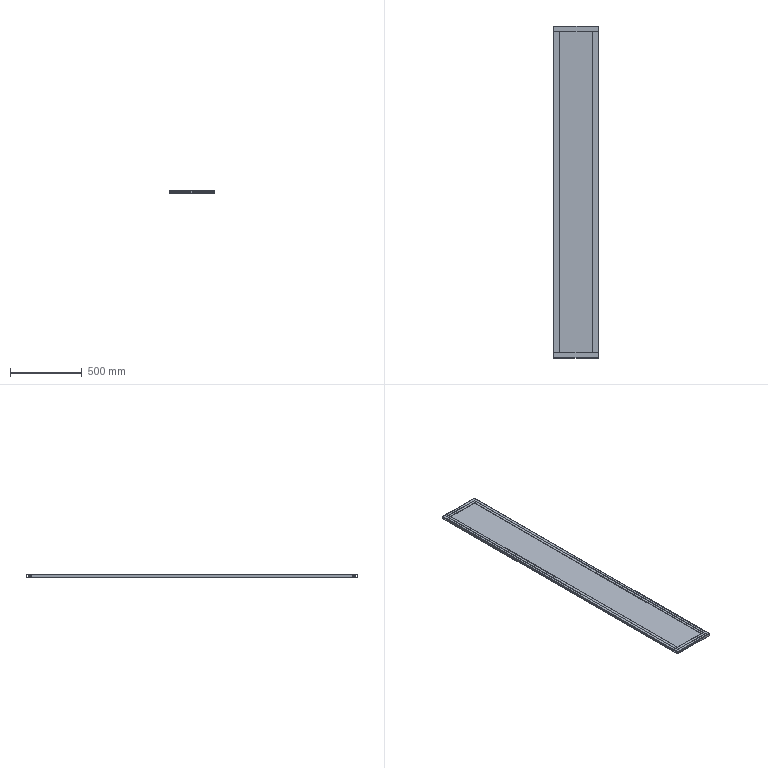Part | SolidWorks | features ICE 1, WeldMemberFeat 1, WeldmentFeature 1 | 5 solids | 158 faces | box 313.5 x 2317 x 18 mm | volume 7344487 mm3 | plane 94 | cylinder 64 | commonest cylinder face diameters 1.1 x24 3.6 x20 5.8 x20